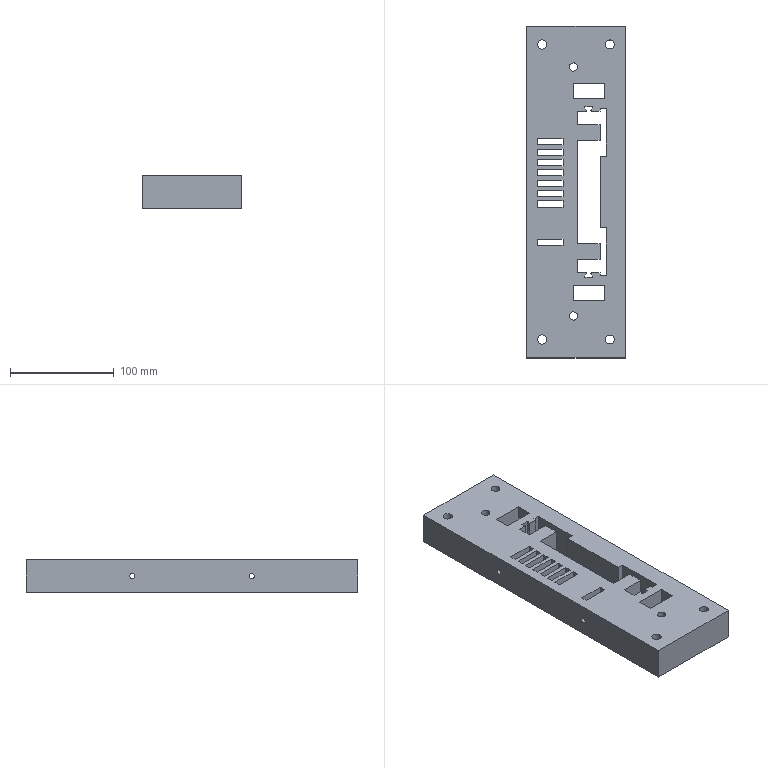Part | STEP file | 1 solid | 111 faces | box 95 x 320 x 31.2 mm | volume 758918 mm3 | plane 80 | cylinder 28 | cone 3 | commonest cylinder face diameters 1 x6 0.52 x4 1.08 x4 5.01 x4 14 x4 8.01 x2